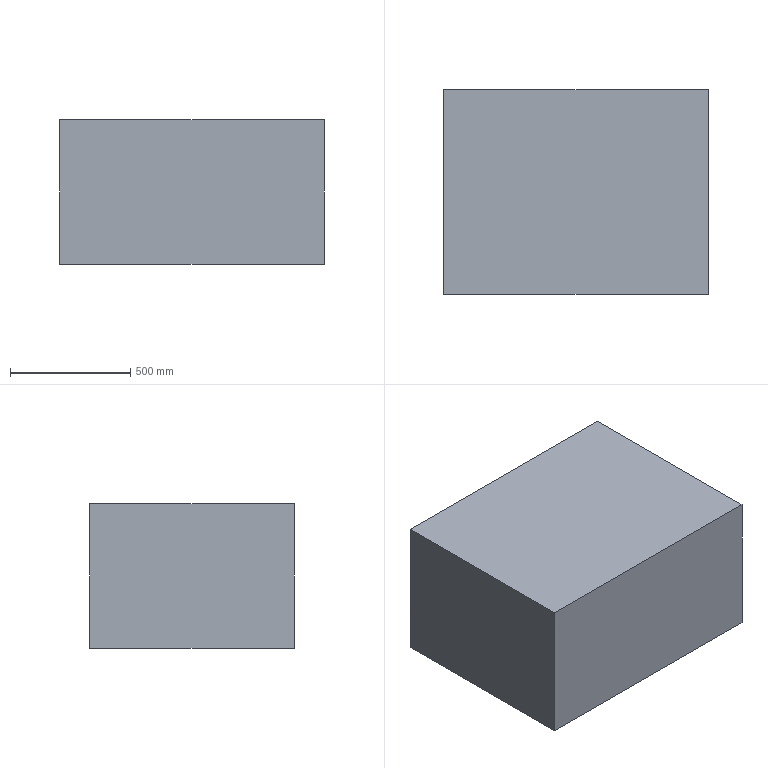Part | SolidWorks | features Extrusion 1 | 1 solid | 6 faces | box 1100 x 850 x 600 mm | volume 561000000 mm3 | plane 6
STEP:
#1=CARTESIAN_POINT('',(0.,850.,0.));
#2=VERTEX_POINT('',#1);
#3=CARTESIAN_POINT('',(0.,0.,0.));
#4=VERTEX_POINT('',#3);
#5=CARTESIAN_POINT('',(0.,0.,0.));
#6=DIRECTION('',(0.,-1.,0.));
#7=VECTOR('',#6,1000.);
#8=LINE('',#5,#7);
#9=EDGE_CURVE('',#2,#4,#8,.T.);
#10=ORIENTED_EDGE('',*,*,#9,.T.);
#11=CARTESIAN_POINT('',(0.,0.,600.));
#12=VERTEX_POINT('',#11);
#13=CARTESIAN_POINT('',(0.,0.,600.));
#14=DIRECTION('',(0.,0.,-1.));
#15=VECTOR('',#14,1000.);
#16=LINE('',#13,#15);
#17=EDGE_CURVE('',#12,#4,#16,.T.);
#18=ORIENTED_EDGE('',*,*,#17,.F.);
#19=CARTESIAN_POINT('',(0.,850.,600.));
#20=VERTEX_POINT('',#19);
#21=CARTESIAN_POINT('',(0.,0.,600.));
#22=DIRECTION('',(0.,-1.,0.));
#23=VECTOR('',#22,1000.);
#24=LINE('',#21,#23);
#25=EDGE_CURVE('',#20,#12,#24,.T.);
#26=ORIENTED_EDGE('',*,*,#25,.F.);
#27=CARTESIAN_POINT('',(0.,850.,600.));
#28=DIRECTION('',(0.,0.,-1.));
#29=VECTOR('',#28,1000.);
#30=LINE('',#27,#29);
#31=EDGE_CURVE('',#20,#2,#30,.T.);
#32=ORIENTED_EDGE('',*,*,#31,.T.);
#33=EDGE_LOOP('',(#10,#18,#26,#32));
#34=FACE_OUTER_BOUND('',#33,.T.);
#35=CARTESIAN_POINT('',(0.,0.,600.));
#36=DIRECTION('',(1.,0.,0.));
#37=DIRECTION('',(0.,0.,-1.));
#38=AXIS2_PLACEMENT_3D('',#35,#36,#37);
#39=PLANE('',#38);
#40=ADVANCED_FACE('',(#34),#39,.F.);
#41=CARTESIAN_POINT('',(1100.,0.,0.));
#42=VERTEX_POINT('',#41);
#43=CARTESIAN_POINT('',(0.,0.,0.));
#44=DIRECTION('',(1.,0.,0.));
#45=VECTOR('',#44,1000.);
#46=LINE('',#43,#45);
#47=EDGE_CURVE('',#4,#42,#46,.T.);
#48=ORIENTED_EDGE('',*,*,#47,.T.);
#49=CARTESIAN_POINT('',(1100.,0.,600.));
#50=VERTEX_POINT('',#49);
#51=CARTESIAN_POINT('',(1100.,0.,600.));
#52=DIRECTION('',(0.,0.,-1.));
#53=VECTOR('',#52,1000.);
#54=LINE('',#51,#53);
#55=EDGE_CURVE('',#50,#42,#54,.T.);
#56=ORIENTED_EDGE('',*,*,#55,.F.);
#57=CARTESIAN_POINT('',(0.,0.,600.));
#58=DIRECTION('',(1.,0.,0.));
#59=VECTOR('',#58,1000.);
#60=LINE('',#57,#59);
#61=EDGE_CURVE('',#12,#50,#60,.T.);
#62=ORIENTED_EDGE('',*,*,#61,.F.);
#63=ORIENTED_EDGE('',*,*,#17,.T.);
#64=EDGE_LOOP('',(#48,#56,#62,#63));
#65=FACE_OUTER_BOUND('',#64,.T.);
#66=CARTESIAN_POINT('',(0.,0.,600.));
#67=DIRECTION('',(0.,1.,0.));
#68=DIRECTION('',(0.,0.,1.));
#69=AXIS2_PLACEMENT_3D('',#66,#67,#68);
#70=PLANE('',#69);
#71=ADVANCED_FACE('',(#65),#70,.F.);
#72=CARTESIAN_POINT('',(1100.,850.,0.));
#73=VERTEX_POINT('',#72);
#74=CARTESIAN_POINT('',(1100.,0.,0.));
#75=DIRECTION('',(0.,1.,0.));
#76=VECTOR('',#75,1000.);
#77=LINE('',#74,#76);
#78=EDGE_CURVE('',#42,#73,#77,.T.);
#79=ORIENTED_EDGE('',*,*,#78,.T.);
#80=CARTESIAN_POINT('',(1100.,850.,600.));
#81=VERTEX_POINT('',#80);
#82=CARTESIAN_POINT('',(1100.,850.,600.));
#83=DIRECTION('',(0.,0.,-1.));
#84=VECTOR('',#83,1000.);
#85=LINE('',#82,#84);
#86=EDGE_CURVE('',#81,#73,#85,.T.);
#87=ORIENTED_EDGE('',*,*,#86,.F.);
#88=CARTESIAN_POINT('',(1100.,0.,600.));
#89=DIRECTION('',(0.,1.,0.));
#90=VECTOR('',#89,1000.);
#91=LINE('',#88,#90);
#92=EDGE_CURVE('',#50,#81,#91,.T.);
#93=ORIENTED_EDGE('',*,*,#92,.F.);
#94=ORIENTED_EDGE('',*,*,#55,.T.);
#95=EDGE_LOOP('',(#79,#87,#93,#94));
#96=FACE_OUTER_BOUND('',#95,.T.);
#97=CARTESIAN_POINT('',(1100.,0.,600.));
#98=DIRECTION('',(-1.,0.,0.));
#99=DIRECTION('',(0.,0.,1.));
#100=AXIS2_PLACEMENT_3D('',#97,#98,#99);
#101=PLANE('',#100);
#102=ADVANCED_FACE('',(#96),#101,.F.);
#103=CARTESIAN_POINT('',(0.,850.,0.));
#104=DIRECTION('',(-1.,0.,0.));
#105=VECTOR('',#104,1000.);
#106=LINE('',#103,#105);
#107=EDGE_CURVE('',#73,#2,#106,.T.);
#108=ORIENTED_EDGE('',*,*,#107,.T.);
#109=ORIENTED_EDGE('',*,*,#31,.F.);
#110=CARTESIAN_POINT('',(0.,850.,600.));
#111=DIRECTION('',(-1.,0.,0.));
#112=VECTOR('',#111,1000.);
#113=LINE('',#110,#112);
#114=EDGE_CURVE('',#81,#20,#113,.T.);
#115=ORIENTED_EDGE('',*,*,#114,.F.);
#116=ORIENTED_EDGE('',*,*,#86,.T.);
#117=EDGE_LOOP('',(#108,#109,#115,#116));
#118=FACE_OUTER_BOUND('',#117,.T.);
#119=CARTESIAN_POINT('',(0.,850.,600.));
#120=DIRECTION('',(0.,-1.,0.));
#121=DIRECTION('',(0.,0.,-1.));
#122=AXIS2_PLACEMENT_3D('',#119,#120,#121);
#123=PLANE('',#122);
#124=ADVANCED_FACE('',(#118),#123,.F.);
#125=ORIENTED_EDGE('',*,*,#25,.T.);
#126=ORIENTED_EDGE('',*,*,#61,.T.);
#127=ORIENTED_EDGE('',*,*,#92,.T.);
#128=ORIENTED_EDGE('',*,*,#114,.T.);
#129=EDGE_LOOP('',(#125,#126,#127,#128));
#130=FACE_OUTER_BOUND('',#129,.T.);
#131=CARTESIAN_POINT('',(0.,0.,600.));
#132=DIRECTION('',(0.,0.,-1.));
#133=DIRECTION('',(-1.,0.,0.));
#134=AXIS2_PLACEMENT_3D('',#131,#132,#133);
#135=PLANE('',#134);
#136=ADVANCED_FACE('',(#130),#135,.F.);
#137=ORIENTED_EDGE('',*,*,#9,.F.);
#138=ORIENTED_EDGE('',*,*,#107,.F.);
#139=ORIENTED_EDGE('',*,*,#78,.F.);
#140=ORIENTED_EDGE('',*,*,#47,.F.);
#141=EDGE_LOOP('',(#137,#138,#139,#140));
#142=FACE_OUTER_BOUND('',#141,.T.);
#143=CARTESIAN_POINT('',(0.,0.,0.));
#144=DIRECTION('',(0.,0.,-1.));
#145=DIRECTION('',(-1.,0.,0.));
#146=AXIS2_PLACEMENT_3D('',#143,#144,#145);
#147=PLANE('',#146);
#148=ADVANCED_FACE('',(#142),#147,.T.);
#149=CLOSED_SHELL('',(#40,#71,#102,#124,#136,#148));
#150=MANIFOLD_SOLID_BREP('',#149);
#151=CARTESIAN_POINT('',(0.,0.,0.));
#152=DIRECTION('',(0.,0.,1.));
#153=DIRECTION('',(1.,0.,0.));
#154=AXIS2_PLACEMENT_3D('',#151,#152,#153);
#155=(LENGTH_UNIT()NAMED_UNIT(*)SI_UNIT(.MILLI.,.METRE.));
#156=UNCERTAINTY_MEASURE_WITH_UNIT(LENGTH_MEASURE(0.00001),#155,'','');
#157=(NAMED_UNIT(*)PLANE_ANGLE_UNIT()SI_UNIT($,.RADIAN.));
#158=(NAMED_UNIT(*)SI_UNIT($,.STERADIAN.)SOLID_ANGLE_UNIT());
#159=(GEOMETRIC_REPRESENTATION_CONTEXT(3)GLOBAL_UNCERTAINTY_ASSIGNED_CONTEXT((#156))GLOBAL_UNIT_ASSIGNED_CONTEXT((#155,#157,#158))REPRESENTATION_CONTEXT('',''));
#160=ADVANCED_BREP_SHAPE_REPRESENTATION('',(#150,#154),#159);